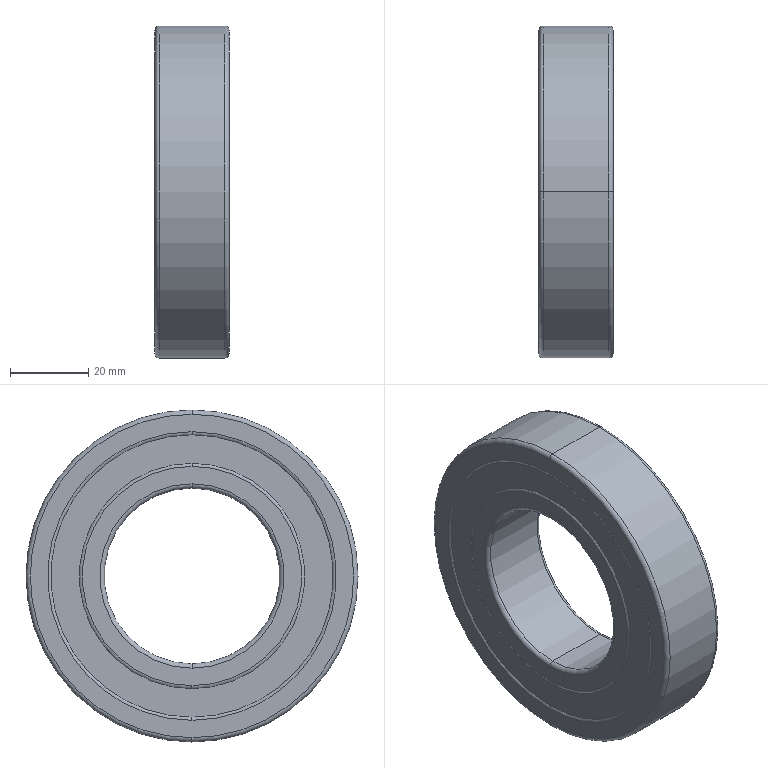Part | SolidWorks | features BaseBody 20 | 20 solids | 212 faces | box 19 x 85 x 85 mm | volume 59594 mm3 | cylinder 74 | sphere 68 | plane 40 | torus 30 | commonest cylinder face diameters 63 x31 67 x31 58.333 x4 71.667 x4 45 x2 85 x2